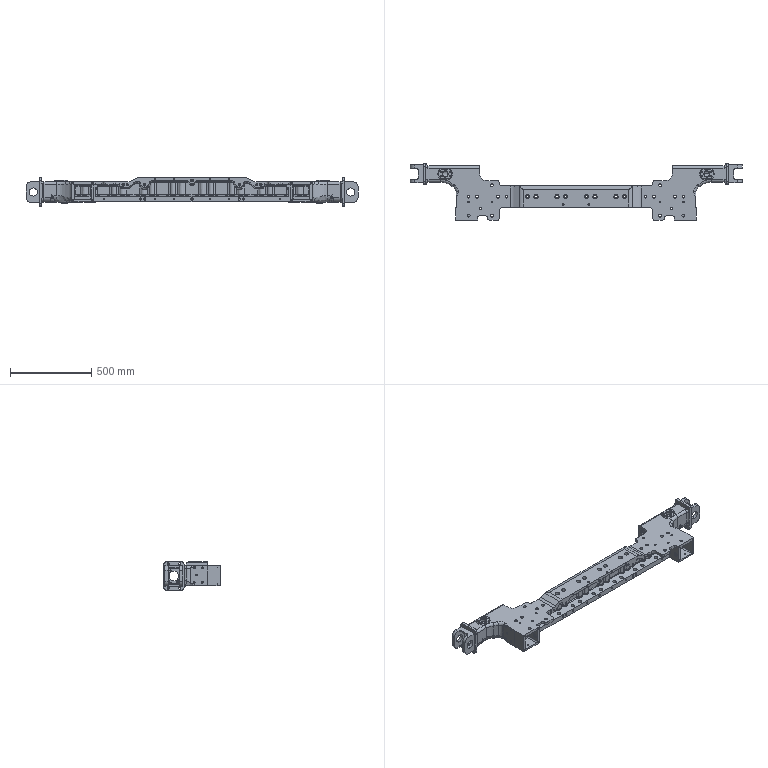Part | SolidWorks | features ICE 2, BaseBody 1, DelFace 1 | 1 solid | 1755 faces | box 2048 x 348 x 175.5 mm | volume 20391465 mm3 | cylinder 782 | cone 358 | spline 304 | plane 265 | torus 40 | sphere 6 | commonest cylinder face diameters 10 x134 30 x90 6.8 x88 17.5 x44 25 x44 27 x42